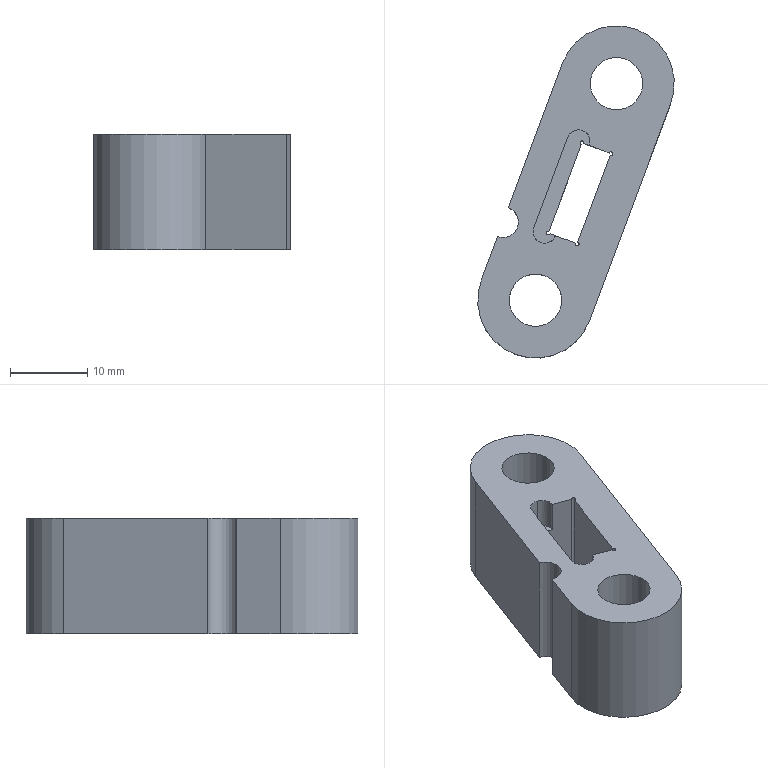Part | NX | features 13 2 | 1 solid | 28 faces | box 25.506 x 43.1 x 15 mm | volume 6274 mm3 | cylinder 15 | plane 13 | commonest cylinder face diameters 0.5 x4 3 x4 6.8 x2 11 x2 15 x2 4.001 x1
STEP:
#1=CARTESIAN_POINT('',(346.445,44.114,15.002));
#2=VERTEX_POINT('',#1);
#3=CARTESIAN_POINT('',(346.445,44.114,0.002032));
#4=VERTEX_POINT('',#3);
#5=CARTESIAN_POINT('',(346.445,44.114,25.));
#6=DIRECTION('',(-0.000000103,0.000000037,-1.));
#7=VECTOR('',#6,1000.);
#8=LINE('',#5,#7);
#9=EDGE_CURVE('',#2,#4,#8,.T.);
#10=ORIENTED_EDGE('',*,*,#9,.F.);
#11=CARTESIAN_POINT('',(353.449,62.847,15.002));
#12=VERTEX_POINT('',#11);
#13=CARTESIAN_POINT('',(344.256,38.26,15.002));
#14=DIRECTION('',(0.3502,0.9367,-0.000000001));
#15=VECTOR('',#14,1000.);
#16=LINE('',#13,#15);
#17=EDGE_CURVE('',#2,#12,#16,.T.);
#18=ORIENTED_EDGE('',*,*,#17,.T.);
#19=CARTESIAN_POINT('',(353.449,62.847,0.002032));
#20=VERTEX_POINT('',#19);
#21=CARTESIAN_POINT('',(353.449,62.847,7.502));
#22=DIRECTION('',(-0.000000103,0.000000037,-1.));
#23=VECTOR('',#22,1000.);
#24=LINE('',#21,#23);
#25=EDGE_CURVE('',#12,#20,#24,.T.);
#26=ORIENTED_EDGE('',*,*,#25,.T.);
#27=CARTESIAN_POINT('',(344.256,38.26,0.002032));
#28=DIRECTION('',(0.3502,0.9367,-0.000000001));
#29=VECTOR('',#28,1000.);
#30=LINE('',#27,#29);
#31=EDGE_CURVE('',#4,#20,#30,.T.);
#32=ORIENTED_EDGE('',*,*,#31,.F.);
#33=EDGE_LOOP('',(#10,#18,#26,#32));
#34=FACE_BOUND('',#33,.T.);
#35=CARTESIAN_POINT('',(344.256,38.26,7.502));
#36=DIRECTION('',(-0.9367,0.3502,0.000000109));
#37=DIRECTION('',(-0.3502,-0.9367,0.00000501));
#38=AXIS2_PLACEMENT_3D('',#35,#36,#37);
#39=PLANE('',#38);
#40=ADVANCED_FACE('',(#34),#39,.T.);
#41=CARTESIAN_POINT('',(356.993,29.494,15.002));
#42=VERTEX_POINT('',#41);
#43=CARTESIAN_POINT('',(367.499,57.594,15.002));
#44=VERTEX_POINT('',#43);
#45=CARTESIAN_POINT('',(358.306,33.007,15.002));
#46=DIRECTION('',(0.3502,0.9367,-0.000000001));
#47=VECTOR('',#46,1000.);
#48=LINE('',#45,#47);
#49=EDGE_CURVE('',#42,#44,#48,.T.);
#50=ORIENTED_EDGE('',*,*,#49,.F.);
#51=CARTESIAN_POINT('',(356.993,29.494,0.00203));
#52=VERTEX_POINT('',#51);
#53=CARTESIAN_POINT('',(356.993,29.494,7.502));
#54=DIRECTION('',(-0.000000103,0.000000037,-1.));
#55=VECTOR('',#54,1000.);
#56=LINE('',#53,#55);
#57=EDGE_CURVE('',#42,#52,#56,.T.);
#58=ORIENTED_EDGE('',*,*,#57,.T.);
#59=CARTESIAN_POINT('',(367.499,57.594,0.00203));
#60=VERTEX_POINT('',#59);
#61=CARTESIAN_POINT('',(358.306,33.007,0.00203));
#62=DIRECTION('',(0.3502,0.9367,-0.000000001));
#63=VECTOR('',#62,1000.);
#64=LINE('',#61,#63);
#65=EDGE_CURVE('',#52,#60,#64,.T.);
#66=ORIENTED_EDGE('',*,*,#65,.T.);
#67=CARTESIAN_POINT('',(367.499,57.594,7.502));
#68=DIRECTION('',(0.000000103,-0.000000037,1.));
#69=VECTOR('',#68,1000.);
#70=LINE('',#67,#69);
#71=EDGE_CURVE('',#60,#44,#70,.T.);
#72=ORIENTED_EDGE('',*,*,#71,.T.);
#73=EDGE_LOOP('',(#50,#58,#66,#72));
#74=FACE_BOUND('',#73,.T.);
#75=CARTESIAN_POINT('',(358.306,33.007,7.502));
#76=DIRECTION('',(-0.9367,0.3502,0.000000109));
#77=DIRECTION('',(-0.3502,-0.9367,0.00000501));
#78=AXIS2_PLACEMENT_3D('',#75,#76,#77);
#79=PLANE('',#78);
#80=ADVANCED_FACE('',(#74),#79,.F.);
#81=CARTESIAN_POINT('',(355.14,39.529,0.002031));
#82=VERTEX_POINT('',#81);
#83=CARTESIAN_POINT('',(351.861,40.754,0.002031));
#84=VERTEX_POINT('',#83);
#85=CARTESIAN_POINT('',(355.373,39.441,0.002031));
#86=DIRECTION('',(-0.9367,0.3502,0.000000109));
#87=VECTOR('',#86,1000.);
#88=LINE('',#85,#87);
#89=EDGE_CURVE('',#82,#84,#88,.T.);
#90=ORIENTED_EDGE('',*,*,#89,.T.);
#91=CARTESIAN_POINT('',(351.861,40.754,11.002));
#92=VERTEX_POINT('',#91);
#93=CARTESIAN_POINT('',(351.861,40.754,5.502));
#94=DIRECTION('',(0.000000104,-0.000000038,1.));
#95=VECTOR('',#94,1000.);
#96=LINE('',#93,#95);
#97=EDGE_CURVE('',#84,#92,#96,.T.);
#98=ORIENTED_EDGE('',*,*,#97,.T.);
#99=CARTESIAN_POINT('',(352.564,40.492,11.002));
#100=VERTEX_POINT('',#99);
#101=CARTESIAN_POINT('',(355.374,39.441,11.002));
#102=DIRECTION('',(0.9367,-0.3502,0.00001998));
#103=VECTOR('',#102,1000.);
#104=LINE('',#101,#103);
#105=EDGE_CURVE('',#92,#100,#104,.T.);
#106=ORIENTED_EDGE('',*,*,#105,.T.);
#107=CARTESIAN_POINT('',(352.564,40.492,15.002));
#108=VERTEX_POINT('',#107);
#109=CARTESIAN_POINT('',(352.564,40.492,11.002));
#110=DIRECTION('',(0.00001871,-0.000006998,-1.));
#111=VECTOR('',#110,1000.);
#112=LINE('',#109,#111);
#113=EDGE_CURVE('',#108,#100,#112,.T.);
#114=ORIENTED_EDGE('',*,*,#113,.F.);
#115=CARTESIAN_POINT('',(355.14,39.529,15.002));
#116=VERTEX_POINT('',#115);
#117=CARTESIAN_POINT('',(355.373,39.441,15.002));
#118=DIRECTION('',(0.9367,-0.3502,-0.000000109));
#119=VECTOR('',#118,1000.);
#120=LINE('',#117,#119);
#121=EDGE_CURVE('',#108,#116,#120,.T.);
#122=ORIENTED_EDGE('',*,*,#121,.T.);
#123=CARTESIAN_POINT('',(355.14,39.529,7.502));
#124=DIRECTION('',(-0.000000103,0.000000037,-1.));
#125=VECTOR('',#124,1000.);
#126=LINE('',#123,#125);
#127=EDGE_CURVE('',#116,#82,#126,.T.);
#128=ORIENTED_EDGE('',*,*,#127,.T.);
#129=EDGE_LOOP('',(#90,#98,#106,#114,#122,#128));
#130=FACE_BOUND('',#129,.T.);
#131=CARTESIAN_POINT('',(355.373,39.441,36.002));
#132=DIRECTION('',(-0.3502,-0.9367,0.000000001));
#133=DIRECTION('',(0.9367,-0.3502,-0.000000109));
#134=AXIS2_PLACEMENT_3D('',#131,#132,#133);
#135=PLANE('',#134);
#136=ADVANCED_FACE('',(#130),#135,.F.);
#137=CARTESIAN_POINT('',(356.941,52.2,11.002));
#138=VERTEX_POINT('',#137);
#139=CARTESIAN_POINT('',(356.239,52.463,11.002));
#140=VERTEX_POINT('',#139);
#141=CARTESIAN_POINT('',(356.005,52.55,11.002));
#142=DIRECTION('',(-0.9367,0.3502,-0.00001998));
#143=VECTOR('',#142,1000.);
#144=LINE('',#141,#143);
#145=EDGE_CURVE('',#138,#140,#144,.T.);
#146=ORIENTED_EDGE('',*,*,#145,.T.);
#147=CARTESIAN_POINT('',(356.239,52.463,0.002031));
#148=VERTEX_POINT('',#147);
#149=CARTESIAN_POINT('',(356.239,52.463,5.502));
#150=DIRECTION('',(-0.000000103,0.000000037,-1.));
#151=VECTOR('',#150,1000.);
#152=LINE('',#149,#151);
#153=EDGE_CURVE('',#140,#148,#152,.T.);
#154=ORIENTED_EDGE('',*,*,#153,.T.);
#155=CARTESIAN_POINT('',(359.517,51.237,0.002031));
#156=VERTEX_POINT('',#155);
#157=CARTESIAN_POINT('',(356.004,52.55,0.002031));
#158=DIRECTION('',(0.9367,-0.3502,-0.000000109));
#159=VECTOR('',#158,1000.);
#160=LINE('',#157,#159);
#161=EDGE_CURVE('',#148,#156,#160,.T.);
#162=ORIENTED_EDGE('',*,*,#161,.T.);
#163=CARTESIAN_POINT('',(359.517,51.237,15.002));
#164=VERTEX_POINT('',#163);
#165=CARTESIAN_POINT('',(359.517,51.237,7.502));
#166=DIRECTION('',(0.000000101,-0.000000037,1.));
#167=VECTOR('',#166,1000.);
#168=LINE('',#165,#167);
#169=EDGE_CURVE('',#156,#164,#168,.T.);
#170=ORIENTED_EDGE('',*,*,#169,.T.);
#171=CARTESIAN_POINT('',(356.941,52.2,15.002));
#172=VERTEX_POINT('',#171);
#173=CARTESIAN_POINT('',(356.004,52.55,15.002));
#174=DIRECTION('',(-0.9367,0.3502,0.000000109));
#175=VECTOR('',#174,1000.);
#176=LINE('',#173,#175);
#177=EDGE_CURVE('',#164,#172,#176,.T.);
#178=ORIENTED_EDGE('',*,*,#177,.T.);
#179=CARTESIAN_POINT('',(356.941,52.2,16.002));
#180=DIRECTION('',(-0.00001871,0.000006998,1.));
#181=VECTOR('',#180,1000.);
#182=LINE('',#179,#181);
#183=EDGE_CURVE('',#138,#172,#182,.T.);
#184=ORIENTED_EDGE('',*,*,#183,.F.);
#185=EDGE_LOOP('',(#146,#154,#162,#170,#178,#184));
#186=FACE_BOUND('',#185,.T.);
#187=CARTESIAN_POINT('',(356.004,52.55,36.002));
#188=DIRECTION('',(0.3502,0.9367,-0.000000001));
#189=DIRECTION('',(-0.9367,0.3502,0.000000109));
#190=AXIS2_PLACEMENT_3D('',#187,#188,#189);
#191=PLANE('',#190);
#192=ADVANCED_FACE('',(#186),#191,.F.);
#193=CARTESIAN_POINT('',(345.044,40.367,15.002));
#194=VERTEX_POINT('',#193);
#195=CARTESIAN_POINT('',(345.744,42.241,15.002));
#196=DIRECTION('',(0.000000103,-0.000000037,1.));
#197=DIRECTION('',(1.,0.,-0.000000103));
#198=AXIS2_PLACEMENT_3D('',#195,#196,#197);
#199=CIRCLE('',#198,2.001);
#200=EDGE_CURVE('',#194,#2,#199,.T.);
#201=ORIENTED_EDGE('',*,*,#200,.F.);
#202=CARTESIAN_POINT('',(342.943,34.747,15.002));
#203=VERTEX_POINT('',#202);
#204=CARTESIAN_POINT('',(344.256,38.26,15.002));
#205=DIRECTION('',(0.3502,0.9367,-0.000000001));
#206=VECTOR('',#205,1000.);
#207=LINE('',#204,#206);
#208=EDGE_CURVE('',#203,#194,#207,.T.);
#209=ORIENTED_EDGE('',*,*,#208,.F.);
#210=CARTESIAN_POINT('',(349.968,32.121,15.002));
#211=DIRECTION('',(0.000000103,-0.000000037,1.));
#212=DIRECTION('',(-0.04361,-0.999,-0.000000033));
#213=AXIS2_PLACEMENT_3D('',#210,#211,#212);
#214=CIRCLE('',#213,7.5);
#215=EDGE_CURVE('',#203,#42,#214,.T.);
#216=ORIENTED_EDGE('',*,*,#215,.T.);
#217=ORIENTED_EDGE('',*,*,#49,.T.);
#218=CARTESIAN_POINT('',(360.474,60.221,15.002));
#219=DIRECTION('',(0.000000103,-0.000000037,1.));
#220=DIRECTION('',(1.,0.,-0.000000103));
#221=AXIS2_PLACEMENT_3D('',#218,#219,#220);
#222=CIRCLE('',#221,7.5);
#223=EDGE_CURVE('',#44,#12,#222,.T.);
#224=ORIENTED_EDGE('',*,*,#223,.T.);
#225=ORIENTED_EDGE('',*,*,#17,.F.);
#226=EDGE_LOOP('',(#201,#209,#216,#217,#224,#225));
#227=FACE_BOUND('',#226,.T.);
#228=CARTESIAN_POINT('',(355.461,39.675,15.002));
#229=VERTEX_POINT('',#228);
#230=CARTESIAN_POINT('',(355.374,39.441,15.002));
#231=DIRECTION('',(-0.000001857,-0.000004654,-1.));
#232=DIRECTION('',(0.999,-0.04361,-0.000001652));
#233=AXIS2_PLACEMENT_3D('',#230,#231,#232);
#234=CIRCLE('',#233,0.25);
#235=EDGE_CURVE('',#229,#116,#234,.T.);
#236=ORIENTED_EDGE('',*,*,#235,.T.);
#237=ORIENTED_EDGE('',*,*,#121,.F.);
#238=CARTESIAN_POINT('',(350.634,39.612,15.002));
#239=VERTEX_POINT('',#238);
#240=CARTESIAN_POINT('',(351.159,41.017,15.002));
#241=DIRECTION('',(0.000000103,-0.000000037,1.));
#242=DIRECTION('',(0.9367,-0.3502,-0.000000109));
#243=AXIS2_PLACEMENT_3D('',#240,#241,#242);
#244=ELLIPSE('',#243,1.5,1.5);
#245=EDGE_CURVE('',#239,#108,#244,.T.);
#246=ORIENTED_EDGE('',*,*,#245,.F.);
#247=CARTESIAN_POINT('',(349.754,41.542,15.002));
#248=VERTEX_POINT('',#247);
#249=CARTESIAN_POINT('',(351.159,41.017,15.002));
#250=DIRECTION('',(0.000000103,-0.000000037,1.));
#251=DIRECTION('',(-0.9367,0.3502,0.000000109));
#252=AXIS2_PLACEMENT_3D('',#249,#250,#251);
#253=ELLIPSE('',#252,1.5,1.5);
#254=EDGE_CURVE('',#248,#239,#253,.T.);
#255=ORIENTED_EDGE('',*,*,#254,.F.);
#256=CARTESIAN_POINT('',(354.131,53.251,15.002));
#257=VERTEX_POINT('',#256);
#258=CARTESIAN_POINT('',(348.003,36.859,15.002));
#259=DIRECTION('',(0.3502,0.9367,-0.000000001));
#260=VECTOR('',#259,1000.);
#261=LINE('',#258,#260);
#262=EDGE_CURVE('',#248,#257,#261,.T.);
#263=ORIENTED_EDGE('',*,*,#262,.T.);
#264=CARTESIAN_POINT('',(356.062,54.13,15.002));
#265=VERTEX_POINT('',#264);
#266=CARTESIAN_POINT('',(355.536,52.725,15.002));
#267=DIRECTION('',(0.000000103,-0.000000037,1.));
#268=DIRECTION('',(0.9367,-0.3502,-0.000000109));
#269=AXIS2_PLACEMENT_3D('',#266,#267,#268);
#270=ELLIPSE('',#269,1.5,1.5);
#271=EDGE_CURVE('',#265,#257,#270,.T.);
#272=ORIENTED_EDGE('',*,*,#271,.F.);
#273=CARTESIAN_POINT('',(355.536,52.725,15.002));
#274=DIRECTION('',(0.000000103,-0.000000037,1.));
#275=DIRECTION('',(-0.9367,0.3502,0.000000109));
#276=AXIS2_PLACEMENT_3D('',#273,#274,#275);
#277=ELLIPSE('',#276,1.5,1.5);
#278=EDGE_CURVE('',#172,#265,#277,.T.);
#279=ORIENTED_EDGE('',*,*,#278,.F.);
#280=ORIENTED_EDGE('',*,*,#177,.F.);
#281=CARTESIAN_POINT('',(359.664,50.915,15.002));
#282=VERTEX_POINT('',#281);
#283=CARTESIAN_POINT('',(359.751,51.15,15.002));
#284=DIRECTION('',(-0.000001857,-0.000004654,-1.));
#285=DIRECTION('',(0.999,-0.04361,-0.000001652));
#286=AXIS2_PLACEMENT_3D('',#283,#284,#285);
#287=CIRCLE('',#286,0.25);
#288=EDGE_CURVE('',#164,#282,#287,.T.);
#289=ORIENTED_EDGE('',*,*,#288,.T.);
#290=CARTESIAN_POINT('',(353.623,34.758,15.002));
#291=DIRECTION('',(0.3502,0.9367,-0.000000001));
#292=VECTOR('',#291,1000.);
#293=LINE('',#290,#292);
#294=EDGE_CURVE('',#229,#282,#293,.T.);
#295=ORIENTED_EDGE('',*,*,#294,.F.);
#296=EDGE_LOOP('',(#236,#237,#246,#255,#263,#272,#279,#280,#289,#295));
#297=FACE_BOUND('',#296,.T.);
#298=CARTESIAN_POINT('',(363.874,60.221,15.002));
#299=VERTEX_POINT('',#298);
#300=CARTESIAN_POINT('',(360.474,60.221,15.002));
#301=DIRECTION('',(0.000000103,-0.000000037,1.));
#302=DIRECTION('',(1.,0.,-0.000000103));
#303=AXIS2_PLACEMENT_3D('',#300,#301,#302);
#304=CIRCLE('',#303,3.4);
#305=EDGE_CURVE('',#299,#299,#304,.T.);
#306=ORIENTED_EDGE('',*,*,#305,.F.);
#307=EDGE_LOOP('',(#306));
#308=FACE_BOUND('',#307,.T.);
#309=CARTESIAN_POINT('',(353.368,32.121,15.002));
#310=VERTEX_POINT('',#309);
#311=CARTESIAN_POINT('',(349.968,32.121,15.002));
#312=DIRECTION('',(-0.000000103,0.000000037,-1.));
#313=DIRECTION('',(1.,0.,-0.000000103));
#314=AXIS2_PLACEMENT_3D('',#311,#312,#313);
#315=CIRCLE('',#314,3.4);
#316=EDGE_CURVE('',#310,#310,#315,.T.);
#317=ORIENTED_EDGE('',*,*,#316,.T.);
#318=EDGE_LOOP('',(#317));
#319=FACE_BOUND('',#318,.T.);
#320=CARTESIAN_POINT('',(351.281,35.633,15.002));
#321=DIRECTION('',(0.000000103,-0.000000037,1.));
#322=DIRECTION('',(-0.04361,-0.999,-0.000000033));
#323=AXIS2_PLACEMENT_3D('',#320,#321,#322);
#324=PLANE('',#323);
#325=ADVANCED_FACE('',(#227,#297,#308,#319),#324,.T.);
#326=CARTESIAN_POINT('',(351.715,41.076,0.002031));
#327=VERTEX_POINT('',#326);
#328=CARTESIAN_POINT('',(355.917,52.316,0.002031));
#329=VERTEX_POINT('',#328);
#330=CARTESIAN_POINT('',(349.876,36.158,0.002031));
#331=DIRECTION('',(0.3502,0.9367,-0.000000001));
#332=VECTOR('',#331,1000.);
#333=LINE('',#330,#332);
#334=EDGE_CURVE('',#327,#329,#333,.T.);
#335=ORIENTED_EDGE('',*,*,#334,.T.);
#336=CARTESIAN_POINT('',(355.917,52.316,11.002));
#337=VERTEX_POINT('',#336);
#338=CARTESIAN_POINT('',(355.917,52.316,5.502));
#339=DIRECTION('',(-0.00001697,0.00001167,1.));
#340=VECTOR('',#339,1000.);
#341=LINE('',#338,#340);
#342=EDGE_CURVE('',#329,#337,#341,.T.);
#343=ORIENTED_EDGE('',*,*,#342,.T.);
#344=CARTESIAN_POINT('',(351.715,41.076,11.002));
#345=VERTEX_POINT('',#344);
#346=CARTESIAN_POINT('',(355.129,50.209,11.002));
#347=DIRECTION('',(0.3502,0.9367,-0.000000001));
#348=VECTOR('',#347,1000.);
#349=LINE('',#346,#348);
#350=EDGE_CURVE('',#345,#337,#349,.T.);
#351=ORIENTED_EDGE('',*,*,#350,.F.);
#352=CARTESIAN_POINT('',(351.715,41.076,5.502));
#353=DIRECTION('',(0.00001696,-0.00001169,-1.));
#354=VECTOR('',#353,1000.);
#355=LINE('',#352,#354);
#356=EDGE_CURVE('',#345,#327,#355,.T.);
#357=ORIENTED_EDGE('',*,*,#356,.T.);
#358=EDGE_LOOP('',(#335,#343,#351,#357));
#359=FACE_BOUND('',#358,.T.);
#360=CARTESIAN_POINT('',(355.129,50.209,36.002));
#361=DIRECTION('',(-0.9367,0.3502,-0.00001998));
#362=DIRECTION('',(-0.3502,-0.9367,0.00000501));
#363=AXIS2_PLACEMENT_3D('',#360,#361,#362);
#364=PLANE('',#363);
#365=ADVANCED_FACE('',(#359),#364,.F.);
#366=CARTESIAN_POINT('',(345.044,40.367,0.002032));
#367=VERTEX_POINT('',#366);
#368=CARTESIAN_POINT('',(345.044,40.367,25.));
#369=DIRECTION('',(0.000000103,-0.000000037,1.));
#370=VECTOR('',#369,1000.);
#371=LINE('',#368,#370);
#372=EDGE_CURVE('',#367,#194,#371,.T.);
#373=ORIENTED_EDGE('',*,*,#372,.F.);
#374=CARTESIAN_POINT('',(342.943,34.747,0.002032));
#375=VERTEX_POINT('',#374);
#376=CARTESIAN_POINT('',(344.256,38.26,0.002032));
#377=DIRECTION('',(0.3502,0.9367,-0.000000001));
#378=VECTOR('',#377,1000.);
#379=LINE('',#376,#378);
#380=EDGE_CURVE('',#375,#367,#379,.T.);
#381=ORIENTED_EDGE('',*,*,#380,.F.);
#382=CARTESIAN_POINT('',(342.943,34.747,7.502));
#383=DIRECTION('',(0.000000103,-0.000000037,1.));
#384=VECTOR('',#383,1000.);
#385=LINE('',#382,#384);
#386=EDGE_CURVE('',#375,#203,#385,.T.);
#387=ORIENTED_EDGE('',*,*,#386,.T.);
#388=ORIENTED_EDGE('',*,*,#208,.T.);
#389=EDGE_LOOP('',(#373,#381,#387,#388));
#390=FACE_BOUND('',#389,.T.);
#391=CARTESIAN_POINT('',(344.256,38.26,7.502));
#392=DIRECTION('',(-0.9367,0.3502,0.000000109));
#393=DIRECTION('',(-0.3502,-0.9367,0.00000501));
#394=AXIS2_PLACEMENT_3D('',#391,#392,#393);
#395=PLANE('',#394);
#396=ADVANCED_FACE('',(#390),#395,.T.);
#397=CARTESIAN_POINT('',(345.744,42.241,0.002032));
#398=DIRECTION('',(-0.000000103,0.000000037,-1.));
#399=DIRECTION('',(-1.,0.,0.000000103));
#400=AXIS2_PLACEMENT_3D('',#397,#398,#399);
#401=CIRCLE('',#400,2.001);
#402=EDGE_CURVE('',#4,#367,#401,.T.);
#403=ORIENTED_EDGE('',*,*,#402,.F.);
#404=ORIENTED_EDGE('',*,*,#31,.T.);
#405=CARTESIAN_POINT('',(360.474,60.221,0.002031));
#406=DIRECTION('',(-0.000000103,0.000000037,-1.));
#407=DIRECTION('',(0.04361,0.999,0.000000033));
#408=AXIS2_PLACEMENT_3D('',#405,#406,#407);
#409=CIRCLE('',#408,7.5);
#410=EDGE_CURVE('',#20,#60,#409,.T.);
#411=ORIENTED_EDGE('',*,*,#410,.T.);
#412=ORIENTED_EDGE('',*,*,#65,.F.);
#413=CARTESIAN_POINT('',(349.968,32.121,0.002031));
#414=DIRECTION('',(-0.000000103,0.000000037,-1.));
#415=DIRECTION('',(-1.,0.,0.000000103));
#416=AXIS2_PLACEMENT_3D('',#413,#414,#415);
#417=CIRCLE('',#416,7.5);
#418=EDGE_CURVE('',#52,#375,#417,.T.);
#419=ORIENTED_EDGE('',*,*,#418,.T.);
#420=ORIENTED_EDGE('',*,*,#380,.T.);
#421=EDGE_LOOP('',(#403,#404,#411,#412,#419,#420));
#422=FACE_BOUND('',#421,.T.);
#423=CARTESIAN_POINT('',(356.005,52.55,0.002031));
#424=DIRECTION('',(-0.000000103,0.000000037,-1.));
#425=DIRECTION('',(0.04361,0.999,0.000000033));
#426=AXIS2_PLACEMENT_3D('',#423,#424,#425);
#427=CIRCLE('',#426,0.25);
#428=EDGE_CURVE('',#329,#148,#427,.T.);
#429=ORIENTED_EDGE('',*,*,#428,.F.);
#430=ORIENTED_EDGE('',*,*,#334,.F.);
#431=CARTESIAN_POINT('',(351.627,40.842,0.002031));
#432=DIRECTION('',(-0.000000103,0.000000037,-1.));
#433=DIRECTION('',(0.04361,0.999,0.000000033));
#434=AXIS2_PLACEMENT_3D('',#431,#432,#433);
#435=CIRCLE('',#434,0.25);
#436=EDGE_CURVE('',#84,#327,#435,.T.);
#437=ORIENTED_EDGE('',*,*,#436,.F.);
#438=ORIENTED_EDGE('',*,*,#89,.F.);
#439=CARTESIAN_POINT('',(355.462,39.675,0.002031));
#440=VERTEX_POINT('',#439);
#441=CARTESIAN_POINT('',(355.374,39.441,0.002031));
#442=DIRECTION('',(-0.000000103,0.000000037,-1.));
#443=DIRECTION('',(0.04361,0.999,0.000000033));
#444=AXIS2_PLACEMENT_3D('',#441,#442,#443);
#445=CIRCLE('',#444,0.25);
#446=EDGE_CURVE('',#440,#82,#445,.T.);
#447=ORIENTED_EDGE('',*,*,#446,.F.);
#448=CARTESIAN_POINT('',(359.664,50.915,0.002031));
#449=VERTEX_POINT('',#448);
#450=CARTESIAN_POINT('',(359.752,51.149,0.002031));
#451=DIRECTION('',(-0.3502,-0.9367,0.000000001));
#452=VECTOR('',#451,1000.);
#453=LINE('',#450,#452);
#454=EDGE_CURVE('',#449,#440,#453,.T.);
#455=ORIENTED_EDGE('',*,*,#454,.F.);
#456=CARTESIAN_POINT('',(359.751,51.149,0.002031));
#457=DIRECTION('',(-0.000000103,0.000000037,-1.));
#458=DIRECTION('',(0.04361,0.999,0.000000033));
#459=AXIS2_PLACEMENT_3D('',#456,#457,#458);
#460=CIRCLE('',#459,0.25);
#461=EDGE_CURVE('',#156,#449,#460,.T.);
#462=ORIENTED_EDGE('',*,*,#461,.F.);
#463=ORIENTED_EDGE('',*,*,#161,.F.);
#464=EDGE_LOOP('',(#429,#430,#437,#438,#447,#455,#462,#463));
#465=FACE_BOUND('',#464,.T.);
#466=CARTESIAN_POINT('',(354.974,60.221,0.002031));
#467=VERTEX_POINT('',#466);
#468=CARTESIAN_POINT('',(360.474,60.221,0.002031));
#469=DIRECTION('',(-0.000000103,0.000000037,-1.));
#470=DIRECTION('',(-1.,0.,0.000000103));
#471=AXIS2_PLACEMENT_3D('',#468,#469,#470);
#472=CIRCLE('',#471,5.5);
#473=EDGE_CURVE('',#467,#467,#472,.T.);
#474=ORIENTED_EDGE('',*,*,#473,.F.);
#475=EDGE_LOOP('',(#474));
#476=FACE_BOUND('',#475,.T.);
#477=CARTESIAN_POINT('',(344.468,32.121,0.002031));
#478=VERTEX_POINT('',#477);
#479=CARTESIAN_POINT('',(349.968,32.121,0.002031));
#480=DIRECTION('',(0.000000103,-0.000000037,1.));
#481=DIRECTION('',(-1.,0.,0.000000103));
#482=AXIS2_PLACEMENT_3D('',#479,#480,#481);
#483=CIRCLE('',#482,5.5);
#484=EDGE_CURVE('',#478,#478,#483,.T.);
#485=ORIENTED_EDGE('',*,*,#484,.T.);
#486=EDGE_LOOP('',(#485));
#487=FACE_BOUND('',#486,.T.);
#488=CARTESIAN_POINT('',(351.281,35.633,0.002031));
#489=DIRECTION('',(-0.000000103,0.000000037,-1.));
#490=DIRECTION('',(0.04361,0.999,0.000000033));
#491=AXIS2_PLACEMENT_3D('',#488,#489,#490);
#492=PLANE('',#491);
#493=ADVANCED_FACE('',(#422,#465,#476,#487),#492,.T.);
#494=ORIENTED_EDGE('',*,*,#215,.F.);
#495=ORIENTED_EDGE('',*,*,#386,.F.);
#496=ORIENTED_EDGE('',*,*,#418,.F.);
#497=ORIENTED_EDGE('',*,*,#57,.F.);
#498=EDGE_LOOP('',(#494,#495,#496,#497));
#499=FACE_BOUND('',#498,.T.);
#500=CARTESIAN_POINT('',(349.968,32.121,7.502));
#501=DIRECTION('',(-0.000000103,0.000000037,-1.));
#502=DIRECTION('',(0.04361,0.999,0.000000033));
#503=AXIS2_PLACEMENT_3D('',#500,#501,#502);
#504=CYLINDRICAL_SURFACE('',#503,7.5);
#505=ADVANCED_FACE('',(#499),#504,.T.);
#506=ORIENTED_EDGE('',*,*,#71,.F.);
#507=ORIENTED_EDGE('',*,*,#410,.F.);
#508=ORIENTED_EDGE('',*,*,#25,.F.);
#509=ORIENTED_EDGE('',*,*,#223,.F.);
#510=EDGE_LOOP('',(#506,#507,#508,#509));
#511=FACE_BOUND('',#510,.T.);
#512=CARTESIAN_POINT('',(360.474,60.221,15.002));
#513=DIRECTION('',(0.000000103,-0.000000037,1.));
#514=DIRECTION('',(-1.,0.,0.000000103));
#515=AXIS2_PLACEMENT_3D('',#512,#513,#514);
#516=CYLINDRICAL_SURFACE('',#515,7.5);
#517=ADVANCED_FACE('',(#511),#516,.T.);
#518=CARTESIAN_POINT('',(353.368,32.121,9.002));
#519=VERTEX_POINT('',#518);
#520=CARTESIAN_POINT('',(349.968,32.121,9.002));
#521=DIRECTION('',(0.000000103,-0.000000037,1.));
#522=DIRECTION('',(1.,0.,-0.000000103));
#523=AXIS2_PLACEMENT_3D('',#520,#521,#522);
#524=CIRCLE('',#523,3.4);
#525=EDGE_CURVE('',#519,#519,#524,.T.);
#526=ORIENTED_EDGE('',*,*,#525,.F.);
#527=EDGE_LOOP('',(#526));
#528=FACE_BOUND('',#527,.T.);
#529=ORIENTED_EDGE('',*,*,#316,.F.);
#530=EDGE_LOOP('',(#529));
#531=FACE_BOUND('',#530,.T.);
#532=CARTESIAN_POINT('',(349.968,32.121,0.002031));
#533=DIRECTION('',(0.000000103,-0.000000037,1.));
#534=DIRECTION('',(0.999,-0.04361,-0.000000104));
#535=AXIS2_PLACEMENT_3D('',#532,#533,#534);
#536=CYLINDRICAL_SURFACE('',#535,3.4);
#537=ADVANCED_FACE('',(#528,#531),#536,.F.);
#538=ORIENTED_EDGE('',*,*,#525,.T.);
#539=EDGE_LOOP('',(#538));
#540=FACE_BOUND('',#539,.T.);
#541=CARTESIAN_POINT('',(355.468,32.121,9.002));
#542=VERTEX_POINT('',#541);
#543=CARTESIAN_POINT('',(349.968,32.121,9.002));
#544=DIRECTION('',(0.000000103,-0.000000037,1.));
#545=DIRECTION('',(1.,0.,-0.000000103));
#546=AXIS2_PLACEMENT_3D('',#543,#544,#545);
#547=CIRCLE('',#546,5.5);
#548=EDGE_CURVE('',#542,#542,#547,.T.);
#549=ORIENTED_EDGE('',*,*,#548,.F.);
#550=EDGE_LOOP('',(#549));
#551=FACE_BOUND('',#550,.T.);
#552=CARTESIAN_POINT('',(349.968,32.121,9.002));
#553=DIRECTION('',(0.000000103,-0.000000037,1.));
#554=DIRECTION('',(-0.04361,-0.999,-0.000000033));
#555=AXIS2_PLACEMENT_3D('',#552,#553,#554);
#556=PLANE('',#555);
#557=ADVANCED_FACE('',(#540,#551),#556,.F.);
#558=ORIENTED_EDGE('',*,*,#548,.T.);
#559=EDGE_LOOP('',(#558));
#560=FACE_BOUND('',#559,.T.);
#561=ORIENTED_EDGE('',*,*,#484,.F.);
#562=EDGE_LOOP('',(#561));
#563=FACE_BOUND('',#562,.T.);
#564=CARTESIAN_POINT('',(349.968,32.121,0.002031));
#565=DIRECTION('',(0.000000103,-0.000000037,1.));
#566=DIRECTION('',(0.999,-0.04361,-0.000000104));
#567=AXIS2_PLACEMENT_3D('',#564,#565,#566);
#568=CYLINDRICAL_SURFACE('',#567,5.5);
#569=ADVANCED_FACE('',(#560,#563),#568,.F.);
#570=CARTESIAN_POINT('',(363.874,60.221,9.002));
#571=VERTEX_POINT('',#570);
#572=CARTESIAN_POINT('',(360.474,60.221,9.002));
#573=DIRECTION('',(-0.000000103,0.000000037,-1.));
#574=DIRECTION('',(1.,0.,-0.000000103));
#575=AXIS2_PLACEMENT_3D('',#572,#573,#574);
#576=CIRCLE('',#575,3.4);
#577=EDGE_CURVE('',#571,#571,#576,.T.);
#578=ORIENTED_EDGE('',*,*,#577,.T.);
#579=EDGE_LOOP('',(#578));
#580=FACE_BOUND('',#579,.T.);
#581=ORIENTED_EDGE('',*,*,#305,.T.);
#582=EDGE_LOOP('',(#581));
#583=FACE_BOUND('',#582,.T.);
#584=CARTESIAN_POINT('',(360.474,60.221,0.002031));
#585=DIRECTION('',(0.000000103,-0.000000037,1.));
#586=DIRECTION('',(0.7826,-0.6225,-0.000000104));
#587=AXIS2_PLACEMENT_3D('',#584,#585,#586);
#588=CYLINDRICAL_SURFACE('',#587,3.4);
#589=ADVANCED_FACE('',(#580,#583),#588,.F.);
#590=ORIENTED_EDGE('',*,*,#577,.F.);
#591=EDGE_LOOP('',(#590));
#592=FACE_BOUND('',#591,.T.);
#593=CARTESIAN_POINT('',(365.974,60.221,9.002));
#594=VERTEX_POINT('',#593);
#595=CARTESIAN_POINT('',(360.474,60.221,9.002));
#596=DIRECTION('',(-0.000000103,0.000000037,-1.));
#597=DIRECTION('',(1.,0.,-0.000000103));
#598=AXIS2_PLACEMENT_3D('',#595,#596,#597);
#599=CIRCLE('',#598,5.5);
#600=EDGE_CURVE('',#594,#594,#599,.T.);
#601=ORIENTED_EDGE('',*,*,#600,.T.);
#602=EDGE_LOOP('',(#601));
#603=FACE_BOUND('',#602,.T.);
#604=CARTESIAN_POINT('',(360.474,60.221,9.002));
#605=DIRECTION('',(0.000000103,-0.000000037,1.));
#606=DIRECTION('',(0.6225,0.7826,-0.000000035));
#607=AXIS2_PLACEMENT_3D('',#604,#605,#606);
#608=PLANE('',#607);
#609=ADVANCED_FACE('',(#592,#603),#608,.F.);
#610=ORIENTED_EDGE('',*,*,#600,.F.);
#611=EDGE_LOOP('',(#610));
#612=FACE_BOUND('',#611,.T.);
#613=ORIENTED_EDGE('',*,*,#473,.T.);
#614=EDGE_LOOP('',(#613));
#615=FACE_BOUND('',#614,.T.);
#616=CARTESIAN_POINT('',(360.474,60.221,0.002031));
#617=DIRECTION('',(0.000000103,-0.000000037,1.));
#618=DIRECTION('',(0.7826,-0.6225,-0.000000104));
#619=AXIS2_PLACEMENT_3D('',#616,#617,#618);
#620=CYLINDRICAL_SURFACE('',#619,5.5);
#621=ADVANCED_FACE('',(#612,#615),#620,.F.);
#622=ORIENTED_EDGE('',*,*,#454,.T.);
#623=CARTESIAN_POINT('',(355.462,39.675,7.502));
#624=DIRECTION('',(-0.00001695,0.00001171,1.));
#625=VECTOR('',#624,1000.);
#626=LINE('',#623,#625);
#627=EDGE_CURVE('',#440,#229,#626,.T.);
#628=ORIENTED_EDGE('',*,*,#627,.T.);
#629=ORIENTED_EDGE('',*,*,#294,.T.);
#630=CARTESIAN_POINT('',(359.664,50.915,7.502));
#631=DIRECTION('',(0.00001696,-0.00001169,-1.));
#632=VECTOR('',#631,1000.);
#633=LINE('',#630,#632);
#634=EDGE_CURVE('',#282,#449,#633,.T.);
#635=ORIENTED_EDGE('',*,*,#634,.T.);
#636=EDGE_LOOP('',(#622,#628,#629,#635));
#637=FACE_BOUND('',#636,.T.);
#638=CARTESIAN_POINT('',(359.751,51.15,36.002));
#639=DIRECTION('',(0.9367,-0.3502,0.00001998));
#640=DIRECTION('',(0.3502,0.9367,-0.00000501));
#641=AXIS2_PLACEMENT_3D('',#638,#639,#640);
#642=PLANE('',#641);
#643=ADVANCED_FACE('',(#637),#642,.F.);
#644=CARTESIAN_POINT('',(356.033,52.799,11.002));
#645=VERTEX_POINT('',#644);
#646=CARTESIAN_POINT('',(356.005,52.55,11.002));
#647=DIRECTION('',(-0.000001857,-0.000004654,-1.));
#648=DIRECTION('',(0.999,-0.04361,-0.000001652));
#649=AXIS2_PLACEMENT_3D('',#646,#647,#648);
#650=CIRCLE('',#649,0.25);
#651=EDGE_CURVE('',#337,#645,#650,.T.);
#652=ORIENTED_EDGE('',*,*,#651,.T.);
#653=CARTESIAN_POINT('',(356.005,52.55,11.002));
#654=DIRECTION('',(0.00001871,-0.000006998,-1.));
#655=DIRECTION('',(-0.999,0.04361,-0.000019));
#656=AXIS2_PLACEMENT_3D('',#653,#654,#655);
#657=CIRCLE('',#656,0.25);
#658=EDGE_CURVE('',#645,#140,#657,.T.);
#659=ORIENTED_EDGE('',*,*,#658,.T.);
#660=ORIENTED_EDGE('',*,*,#145,.F.);
#661=CARTESIAN_POINT('',(356.062,54.13,11.002));
#662=VERTEX_POINT('',#661);
#663=CARTESIAN_POINT('',(355.536,52.725,11.002));
#664=DIRECTION('',(0.00001871,-0.000006998,-1.));
#665=DIRECTION('',(0.999,-0.04361,0.000019));
#666=AXIS2_PLACEMENT_3D('',#663,#664,#665);
#667=CIRCLE('',#666,1.5);
#668=EDGE_CURVE('',#662,#138,#667,.T.);
#669=ORIENTED_EDGE('',*,*,#668,.F.);
#670=CARTESIAN_POINT('',(354.131,53.251,11.002));
#671=VERTEX_POINT('',#670);
#672=CARTESIAN_POINT('',(355.536,52.725,11.002));
#673=DIRECTION('',(0.00001871,-0.000006998,-1.));
#674=DIRECTION('',(0.999,-0.04361,0.000019));
#675=AXIS2_PLACEMENT_3D('',#672,#673,#674);
#676=CIRCLE('',#675,1.5);
#677=EDGE_CURVE('',#671,#662,#676,.T.);
#678=ORIENTED_EDGE('',*,*,#677,.F.);
#679=CARTESIAN_POINT('',(349.754,41.542,11.002));
#680=VERTEX_POINT('',#679);
#681=CARTESIAN_POINT('',(352.818,49.738,11.002));
#682=DIRECTION('',(0.3502,0.9367,-0.000000001));
#683=VECTOR('',#682,1000.);
#684=LINE('',#681,#683);
#685=EDGE_CURVE('',#680,#671,#684,.T.);
#686=ORIENTED_EDGE('',*,*,#685,.F.);
#687=CARTESIAN_POINT('',(350.634,39.612,11.002));
#688=VERTEX_POINT('',#687);
#689=CARTESIAN_POINT('',(351.159,41.017,11.002));
#690=DIRECTION('',(0.00001871,-0.000006998,-1.));
#691=DIRECTION('',(0.999,-0.04361,0.000019));
#692=AXIS2_PLACEMENT_3D('',#689,#690,#691);
#693=CIRCLE('',#692,1.5);
#694=EDGE_CURVE('',#688,#680,#693,.T.);
#695=ORIENTED_EDGE('',*,*,#694,.F.);
#696=CARTESIAN_POINT('',(351.159,41.017,11.002));
#697=DIRECTION('',(0.00001871,-0.000006998,-1.));
#698=DIRECTION('',(0.999,-0.04361,0.000019));
#699=AXIS2_PLACEMENT_3D('',#696,#697,#698);
#700=CIRCLE('',#699,1.5);
#701=EDGE_CURVE('',#100,#688,#700,.T.);
#702=ORIENTED_EDGE('',*,*,#701,.F.);
#703=ORIENTED_EDGE('',*,*,#105,.F.);
#704=CARTESIAN_POINT('',(351.599,40.593,11.002));
#705=VERTEX_POINT('',#704);
#706=CARTESIAN_POINT('',(351.627,40.842,11.002));
#707=DIRECTION('',(-0.000001857,-0.000004654,-1.));
#708=DIRECTION('',(0.999,-0.04361,-0.000001652));
#709=AXIS2_PLACEMENT_3D('',#706,#707,#708);
#710=CIRCLE('',#709,0.25);
#711=EDGE_CURVE('',#92,#705,#710,.T.);
#712=ORIENTED_EDGE('',*,*,#711,.T.);
#713=CARTESIAN_POINT('',(351.627,40.842,11.002));
#714=DIRECTION('',(0.00001871,-0.000006998,-1.));
#715=DIRECTION('',(-0.999,0.04361,-0.000019));
#716=AXIS2_PLACEMENT_3D('',#713,#714,#715);
#717=CIRCLE('',#716,0.25);
#718=EDGE_CURVE('',#705,#345,#717,.T.);
#719=ORIENTED_EDGE('',*,*,#718,.T.);
#720=ORIENTED_EDGE('',*,*,#350,.T.);
#721=EDGE_LOOP('',(#652,#659,#660,#669,#678,#686,#695,#702,#703,#712,#719,#720));
#722=FACE_BOUND('',#721,.T.);
#723=CARTESIAN_POINT('',(356.565,48.337,11.002));
#724=DIRECTION('',(0.00001871,-0.000006998,-1.));
#725=DIRECTION('',(0.9367,-0.3502,0.00001998));
#726=AXIS2_PLACEMENT_3D('',#723,#724,#725);
#727=PLANE('',#726);
#728=ADVANCED_FACE('',(#722),#727,.F.);
#729=CARTESIAN_POINT('',(349.754,41.542,-0.3468));
#730=DIRECTION('',(0.00001871,-0.000006998,-1.));
#731=VECTOR('',#730,1000.);
#732=LINE('',#729,#731);
#733=EDGE_CURVE('',#248,#680,#732,.T.);
#734=ORIENTED_EDGE('',*,*,#733,.T.);
#735=ORIENTED_EDGE('',*,*,#685,.T.);
#736=CARTESIAN_POINT('',(354.132,53.251,-0.3448));
#737=DIRECTION('',(-0.00001871,0.000006998,1.));
#738=VECTOR('',#737,1000.);
#739=LINE('',#736,#738);
#740=EDGE_CURVE('',#671,#257,#739,.T.);
#741=ORIENTED_EDGE('',*,*,#740,.T.);
#742=ORIENTED_EDGE('',*,*,#262,.F.);
#743=EDGE_LOOP('',(#734,#735,#741,#742));
#744=FACE_BOUND('',#743,.T.);
#745=CARTESIAN_POINT('',(353.256,50.909,-0.3468));
#746=DIRECTION('',(0.9367,-0.3502,0.00001998));
#747=DIRECTION('',(0.3502,0.9367,-0.000000001));
#748=AXIS2_PLACEMENT_3D('',#745,#746,#747);
#749=PLANE('',#748);
#750=ADVANCED_FACE('',(#744),#749,.T.);
#751=ORIENTED_EDGE('',*,*,#245,.T.);
#752=ORIENTED_EDGE('',*,*,#113,.T.);
#753=ORIENTED_EDGE('',*,*,#701,.T.);
#754=CARTESIAN_POINT('',(350.634,39.612,16.002));
#755=DIRECTION('',(0.00001871,-0.000006998,-1.));
#756=VECTOR('',#755,1000.);
#757=LINE('',#754,#756);
#758=EDGE_CURVE('',#239,#688,#757,.T.);
#759=ORIENTED_EDGE('',*,*,#758,.F.);
#760=EDGE_LOOP('',(#751,#752,#753,#759));
#761=FACE_BOUND('',#760,.T.);
#762=CARTESIAN_POINT('',(351.159,41.017,-0.3524));
#763=DIRECTION('',(0.00001871,-0.000006998,-1.));
#764=DIRECTION('',(-0.999,0.04361,-0.000019));
#765=AXIS2_PLACEMENT_3D('',#762,#763,#764);
#766=CYLINDRICAL_SURFACE('',#765,1.5);
#767=ADVANCED_FACE('',(#761),#766,.F.);
#768=ORIENTED_EDGE('',*,*,#254,.T.);
#769=ORIENTED_EDGE('',*,*,#758,.T.);
#770=ORIENTED_EDGE('',*,*,#694,.T.);
#771=ORIENTED_EDGE('',*,*,#733,.F.);
#772=EDGE_LOOP('',(#768,#769,#770,#771));
#773=FACE_BOUND('',#772,.T.);
#774=CARTESIAN_POINT('',(351.159,41.017,-0.3468));
#775=DIRECTION('',(-0.00001871,0.000006998,1.));
#776=DIRECTION('',(0.999,-0.04361,0.000019));
#777=AXIS2_PLACEMENT_3D('',#774,#775,#776);
#778=CYLINDRICAL_SURFACE('',#777,1.5);
#779=ADVANCED_FACE('',(#773),#778,.F.);
#780=ORIENTED_EDGE('',*,*,#278,.T.);
#781=CARTESIAN_POINT('',(356.062,54.13,11.002));
#782=DIRECTION('',(-0.00001871,0.000006998,1.));
#783=VECTOR('',#782,1000.);
#784=LINE('',#781,#783);
#785=EDGE_CURVE('',#662,#265,#784,.T.);
#786=ORIENTED_EDGE('',*,*,#785,.F.);
#787=ORIENTED_EDGE('',*,*,#668,.T.);
#788=ORIENTED_EDGE('',*,*,#183,.T.);
#789=EDGE_LOOP('',(#780,#786,#787,#788));
#790=FACE_BOUND('',#789,.T.);
#791=CARTESIAN_POINT('',(355.537,52.725,-0.3468));
#792=DIRECTION('',(-0.00001871,0.000006998,1.));
#793=DIRECTION('',(0.999,-0.04361,0.000019));
#794=AXIS2_PLACEMENT_3D('',#791,#792,#793);
#795=CYLINDRICAL_SURFACE('',#794,1.5);
#796=ADVANCED_FACE('',(#790),#795,.F.);
#797=ORIENTED_EDGE('',*,*,#271,.T.);
#798=ORIENTED_EDGE('',*,*,#740,.F.);
#799=ORIENTED_EDGE('',*,*,#677,.T.);
#800=ORIENTED_EDGE('',*,*,#785,.T.);
#801=EDGE_LOOP('',(#797,#798,#799,#800));
#802=FACE_BOUND('',#801,.T.);
#803=CARTESIAN_POINT('',(355.537,52.725,-0.3448));
#804=DIRECTION('',(0.00001871,-0.000006998,-1.));
#805=DIRECTION('',(-0.999,0.04361,-0.000019));
#806=AXIS2_PLACEMENT_3D('',#803,#804,#805);
#807=CYLINDRICAL_SURFACE('',#806,1.5);
#808=ADVANCED_FACE('',(#802),#807,.F.);
#809=ORIENTED_EDGE('',*,*,#461,.T.);
#810=ORIENTED_EDGE('',*,*,#634,.F.);
#811=ORIENTED_EDGE('',*,*,#288,.F.);
#812=ORIENTED_EDGE('',*,*,#169,.F.);
#813=EDGE_LOOP('',(#809,#810,#811,#812));
#814=FACE_BOUND('',#813,.T.);
#815=CARTESIAN_POINT('',(359.751,51.15,15.002));
#816=DIRECTION('',(-0.000001857,-0.000004654,-1.));
#817=DIRECTION('',(0.999,-0.04361,-0.000001652));
#818=AXIS2_PLACEMENT_3D('',#815,#816,#817);
#819=CYLINDRICAL_SURFACE('',#818,0.25);
#820=ADVANCED_FACE('',(#814),#819,.F.);
#821=ORIENTED_EDGE('',*,*,#235,.F.);
#822=ORIENTED_EDGE('',*,*,#627,.F.);
#823=ORIENTED_EDGE('',*,*,#446,.T.);
#824=ORIENTED_EDGE('',*,*,#127,.F.);
#825=EDGE_LOOP('',(#821,#822,#823,#824));
#826=FACE_BOUND('',#825,.T.);
#827=CARTESIAN_POINT('',(355.374,39.441,15.002));
#828=DIRECTION('',(-0.000001857,-0.000004654,-1.));
#829=DIRECTION('',(0.999,-0.04361,-0.000001652));
#830=AXIS2_PLACEMENT_3D('',#827,#828,#829);
#831=CYLINDRICAL_SURFACE('',#830,0.25);
#832=ADVANCED_FACE('',(#826),#831,.F.);
#833=ORIENTED_EDGE('',*,*,#436,.T.);
#834=ORIENTED_EDGE('',*,*,#356,.F.);
#835=ORIENTED_EDGE('',*,*,#718,.F.);
#836=ORIENTED_EDGE('',*,*,#711,.F.);
#837=ORIENTED_EDGE('',*,*,#97,.F.);
#838=EDGE_LOOP('',(#833,#834,#835,#836,#837));
#839=FACE_BOUND('',#838,.T.);
#840=CARTESIAN_POINT('',(351.627,40.842,11.002));
#841=DIRECTION('',(-0.000001857,-0.000004654,-1.));
#842=DIRECTION('',(0.999,-0.04361,-0.000001652));
#843=AXIS2_PLACEMENT_3D('',#840,#841,#842);
#844=CYLINDRICAL_SURFACE('',#843,0.25);
#845=ADVANCED_FACE('',(#839),#844,.F.);
#846=ORIENTED_EDGE('',*,*,#658,.F.);
#847=ORIENTED_EDGE('',*,*,#651,.F.);
#848=ORIENTED_EDGE('',*,*,#342,.F.);
#849=ORIENTED_EDGE('',*,*,#428,.T.);
#850=ORIENTED_EDGE('',*,*,#153,.F.);
#851=EDGE_LOOP('',(#846,#847,#848,#849,#850));
#852=FACE_BOUND('',#851,.T.);
#853=CARTESIAN_POINT('',(356.005,52.55,11.002));
#854=DIRECTION('',(-0.000001857,-0.000004654,-1.));
#855=DIRECTION('',(0.999,-0.04361,-0.000001652));
#856=AXIS2_PLACEMENT_3D('',#853,#854,#855);
#857=CYLINDRICAL_SURFACE('',#856,0.25);
#858=ADVANCED_FACE('',(#852),#857,.F.);
#859=ORIENTED_EDGE('',*,*,#200,.T.);
#860=ORIENTED_EDGE('',*,*,#9,.T.);
#861=ORIENTED_EDGE('',*,*,#402,.T.);
#862=ORIENTED_EDGE('',*,*,#372,.T.);
#863=EDGE_LOOP('',(#859,#860,#861,#862));
#864=FACE_BOUND('',#863,.T.);
#865=CARTESIAN_POINT('',(345.744,42.241,25.));
#866=DIRECTION('',(-0.000000103,0.000000037,-1.));
#867=DIRECTION('',(0.7663,-0.6425,-0.000000103));
#868=AXIS2_PLACEMENT_3D('',#865,#866,#867);
#869=CYLINDRICAL_SURFACE('',#868,2.001);
#870=ADVANCED_FACE('',(#864),#869,.F.);
#871=CLOSED_SHELL('',(#40,#80,#136,#192,#325,#365,#396,#493,#505,#517,#537,#557,#569,#589,#609,#621,#643,#728,#750,#767,#779,#796,#808,#820,#832,#845,#858,#870));
#872=MANIFOLD_SOLID_BREP('',#871);
#873=(LENGTH_UNIT()NAMED_UNIT(*)SI_UNIT(.MILLI.,.METRE.));
#874=UNCERTAINTY_MEASURE_WITH_UNIT(LENGTH_MEASURE(0.00001),#873,'','');
#875=(NAMED_UNIT(*)PLANE_ANGLE_UNIT()SI_UNIT($,.RADIAN.));
#876=(NAMED_UNIT(*)SI_UNIT($,.STERADIAN.)SOLID_ANGLE_UNIT());
#877=(GEOMETRIC_REPRESENTATION_CONTEXT(3)GLOBAL_UNCERTAINTY_ASSIGNED_CONTEXT((#874))GLOBAL_UNIT_ASSIGNED_CONTEXT((#873,#875,#876))REPRESENTATION_CONTEXT('',''));
#878=ADVANCED_BREP_SHAPE_REPRESENTATION('',(#872),#877);